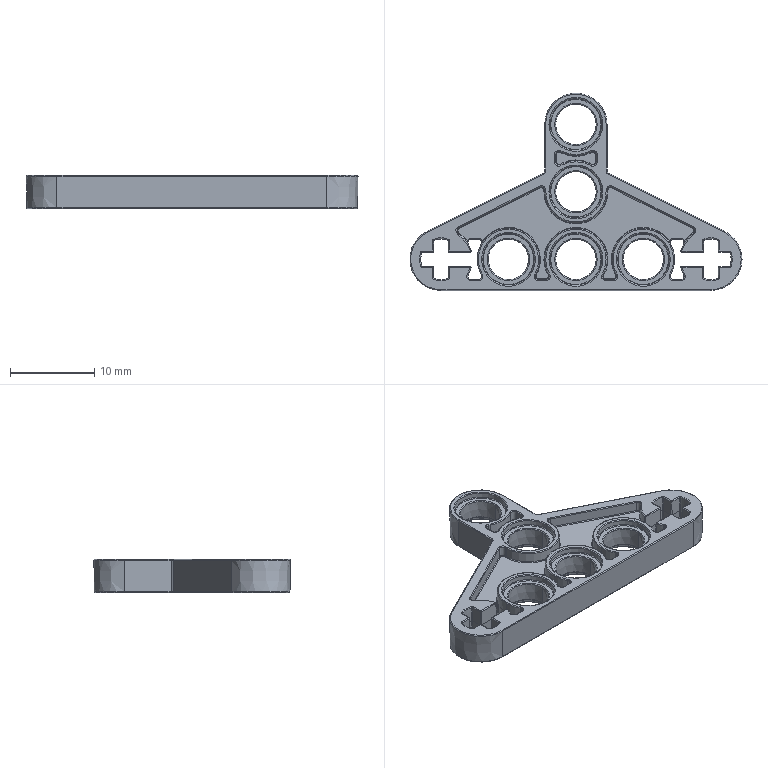Part | STEP file | Moulded part | 1 solid | 698 faces | box 39.381 x 23.386 x 3.923 mm | volume 972.135 mm3 | torus 260 | cone 176 | cylinder 101 | plane 85 | spline 64 | sphere 12 | commonest cylinder face diameters 0.201 x101